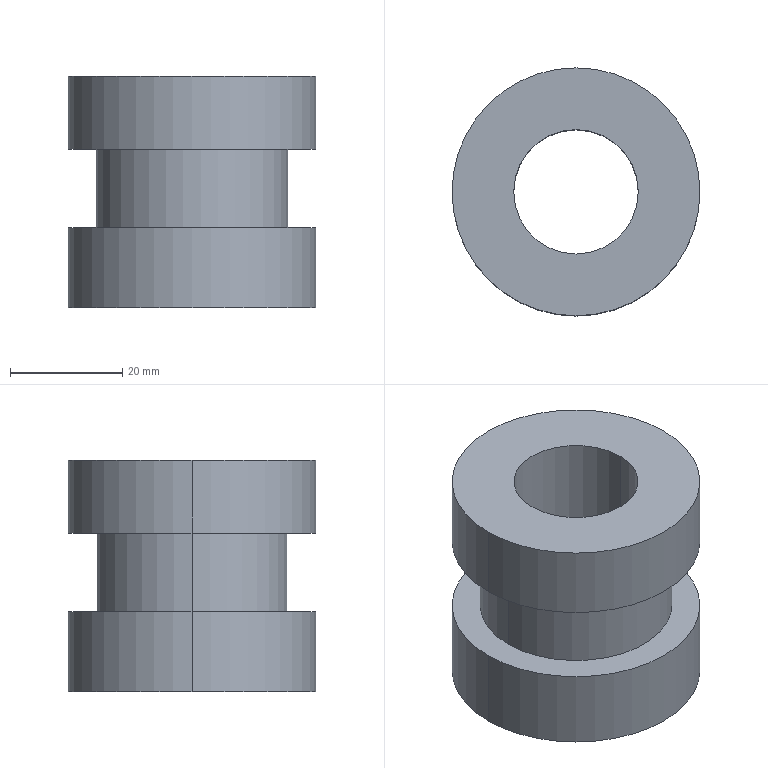Part | STEP file | 4-20.sldasm-Part-109 | 1 solid | 12 faces | box 44.22 x 44.22 x 41.275 mm | volume 38759 mm3 | cylinder 8 | plane 4 | commonest cylinder face diameters 44.22 x4 22.22 x2 34.22 x2
STEP:
#1=CARTESIAN_POINT('',(22.11,-584.45,-181.275));
#2=VERTEX_POINT('',#1);
#3=CARTESIAN_POINT('',(-22.11,-584.45,-181.275));
#4=VERTEX_POINT('',#3);
#5=CARTESIAN_POINT('',(0.,-584.45,-181.275));
#6=DIRECTION('',(0.,0.,1.));
#7=DIRECTION('',(1.,0.,0.));
#8=AXIS2_PLACEMENT_3D('',#5,#6,#7);
#9=CIRCLE('',#8,22.11);
#10=EDGE_CURVE('',#2,#4,#9,.T.);
#11=ORIENTED_EDGE('',*,*,#10,.T.);
#12=CARTESIAN_POINT('',(-22.11,-584.45,-167.));
#13=VERTEX_POINT('',#12);
#14=CARTESIAN_POINT('',(-22.11,-584.45,-179.));
#15=DIRECTION('',(0.,0.,1.));
#16=VECTOR('',#15,1000.);
#17=LINE('',#14,#16);
#18=EDGE_CURVE('',#4,#13,#17,.T.);
#19=ORIENTED_EDGE('',*,*,#18,.T.);
#20=CARTESIAN_POINT('',(22.11,-584.45,-167.));
#21=VERTEX_POINT('',#20);
#22=CARTESIAN_POINT('',(0.,-584.45,-167.));
#23=DIRECTION('',(0.,0.,1.));
#24=DIRECTION('',(-1.,0.,0.));
#25=AXIS2_PLACEMENT_3D('',#22,#23,#24);
#26=CIRCLE('',#25,22.11);
#27=EDGE_CURVE('',#21,#13,#26,.T.);
#28=ORIENTED_EDGE('',*,*,#27,.F.);
#29=CARTESIAN_POINT('',(22.11,-584.45,-179.));
#30=DIRECTION('',(0.,0.,1.));
#31=VECTOR('',#30,1000.);
#32=LINE('',#29,#31);
#33=EDGE_CURVE('',#2,#21,#32,.T.);
#34=ORIENTED_EDGE('',*,*,#33,.F.);
#35=EDGE_LOOP('',(#11,#19,#28,#34));
#36=FACE_OUTER_BOUND('',#35,.T.);
#37=CARTESIAN_POINT('',(0.,-584.45,-179.));
#38=DIRECTION('',(0.,0.,1.));
#39=DIRECTION('',(1.,0.,0.));
#40=AXIS2_PLACEMENT_3D('',#37,#38,#39);
#41=CYLINDRICAL_SURFACE('',#40,22.11);
#42=ADVANCED_FACE('',(#36),#41,.T.);
#43=CARTESIAN_POINT('',(-22.11,-584.45,-140.));
#44=VERTEX_POINT('',#43);
#45=CARTESIAN_POINT('',(22.11,-584.45,-140.));
#46=VERTEX_POINT('',#45);
#47=CARTESIAN_POINT('',(0.,-584.45,-140.));
#48=DIRECTION('',(0.,0.,-1.));
#49=DIRECTION('',(1.,0.,0.));
#50=AXIS2_PLACEMENT_3D('',#47,#48,#49);
#51=CIRCLE('',#50,22.11);
#52=EDGE_CURVE('',#44,#46,#51,.T.);
#53=ORIENTED_EDGE('',*,*,#52,.T.);
#54=CARTESIAN_POINT('',(22.11,-584.45,-153.));
#55=VERTEX_POINT('',#54);
#56=CARTESIAN_POINT('',(22.11,-584.45,-139.));
#57=DIRECTION('',(0.,0.,-1.));
#58=VECTOR('',#57,1000.);
#59=LINE('',#56,#58);
#60=EDGE_CURVE('',#46,#55,#59,.T.);
#61=ORIENTED_EDGE('',*,*,#60,.T.);
#62=CARTESIAN_POINT('',(-22.11,-584.45,-153.));
#63=VERTEX_POINT('',#62);
#64=CARTESIAN_POINT('',(0.,-584.45,-153.));
#65=DIRECTION('',(0.,0.,-1.));
#66=DIRECTION('',(1.,0.,0.));
#67=AXIS2_PLACEMENT_3D('',#64,#65,#66);
#68=CIRCLE('',#67,22.11);
#69=EDGE_CURVE('',#63,#55,#68,.T.);
#70=ORIENTED_EDGE('',*,*,#69,.F.);
#71=CARTESIAN_POINT('',(-22.11,-584.45,-139.));
#72=DIRECTION('',(0.,0.,-1.));
#73=VECTOR('',#72,1000.);
#74=LINE('',#71,#73);
#75=EDGE_CURVE('',#44,#63,#74,.T.);
#76=ORIENTED_EDGE('',*,*,#75,.F.);
#77=EDGE_LOOP('',(#53,#61,#70,#76));
#78=FACE_OUTER_BOUND('',#77,.T.);
#79=CARTESIAN_POINT('',(0.,-584.45,-139.));
#80=DIRECTION('',(0.,0.,-1.));
#81=DIRECTION('',(-1.,0.,0.));
#82=AXIS2_PLACEMENT_3D('',#79,#80,#81);
#83=CYLINDRICAL_SURFACE('',#82,22.11);
#84=ADVANCED_FACE('',(#78),#83,.T.);
#85=CARTESIAN_POINT('',(-11.11,-584.45,-181.275));
#86=VERTEX_POINT('',#85);
#87=CARTESIAN_POINT('',(11.11,-584.45,-181.275));
#88=VERTEX_POINT('',#87);
#89=CARTESIAN_POINT('',(0.,-584.45,-181.275));
#90=DIRECTION('',(0.,0.,1.));
#91=DIRECTION('',(1.,0.,0.));
#92=AXIS2_PLACEMENT_3D('',#89,#90,#91);
#93=CIRCLE('',#92,11.11);
#94=EDGE_CURVE('',#86,#88,#93,.T.);
#95=ORIENTED_EDGE('',*,*,#94,.F.);
#96=CARTESIAN_POINT('',(-11.11,-584.45,-140.));
#97=VERTEX_POINT('',#96);
#98=CARTESIAN_POINT('',(-11.11,-584.45,-168.9));
#99=DIRECTION('',(0.,0.,1.));
#100=VECTOR('',#99,1000.);
#101=LINE('',#98,#100);
#102=EDGE_CURVE('',#86,#97,#101,.T.);
#103=ORIENTED_EDGE('',*,*,#102,.T.);
#104=CARTESIAN_POINT('',(11.11,-584.45,-140.));
#105=VERTEX_POINT('',#104);
#106=CARTESIAN_POINT('',(0.,-584.45,-140.));
#107=DIRECTION('',(0.,0.,1.));
#108=DIRECTION('',(1.,0.,0.));
#109=AXIS2_PLACEMENT_3D('',#106,#107,#108);
#110=CIRCLE('',#109,11.11);
#111=EDGE_CURVE('',#97,#105,#110,.T.);
#112=ORIENTED_EDGE('',*,*,#111,.T.);
#113=CARTESIAN_POINT('',(11.11,-584.45,-168.9));
#114=DIRECTION('',(0.,0.,1.));
#115=VECTOR('',#114,1000.);
#116=LINE('',#113,#115);
#117=EDGE_CURVE('',#88,#105,#116,.T.);
#118=ORIENTED_EDGE('',*,*,#117,.F.);
#119=EDGE_LOOP('',(#95,#103,#112,#118));
#120=FACE_OUTER_BOUND('',#119,.T.);
#121=CARTESIAN_POINT('',(0.,-584.45,-168.9));
#122=DIRECTION('',(0.,0.,1.));
#123=DIRECTION('',(1.,0.,0.));
#124=AXIS2_PLACEMENT_3D('',#121,#122,#123);
#125=CYLINDRICAL_SURFACE('',#124,11.11);
#126=ADVANCED_FACE('',(#120),#125,.F.);
#127=CARTESIAN_POINT('',(-17.11,-584.45,-167.));
#128=VERTEX_POINT('',#127);
#129=CARTESIAN_POINT('',(17.11,-584.45,-167.));
#130=VERTEX_POINT('',#129);
#131=CARTESIAN_POINT('',(0.,-584.45,-167.));
#132=DIRECTION('',(0.,0.,-1.));
#133=DIRECTION('',(-1.,0.,0.));
#134=AXIS2_PLACEMENT_3D('',#131,#132,#133);
#135=CIRCLE('',#134,17.11);
#136=EDGE_CURVE('',#128,#130,#135,.T.);
#137=ORIENTED_EDGE('',*,*,#136,.F.);
#138=CARTESIAN_POINT('',(-17.11,-584.45,-153.));
#139=VERTEX_POINT('',#138);
#140=CARTESIAN_POINT('',(-17.11,-584.45,-168.9));
#141=DIRECTION('',(0.,0.,1.));
#142=VECTOR('',#141,1000.);
#143=LINE('',#140,#142);
#144=EDGE_CURVE('',#128,#139,#143,.T.);
#145=ORIENTED_EDGE('',*,*,#144,.T.);
#146=CARTESIAN_POINT('',(17.11,-584.45,-153.));
#147=VERTEX_POINT('',#146);
#148=CARTESIAN_POINT('',(0.,-584.45,-153.));
#149=DIRECTION('',(0.,0.,1.));
#150=DIRECTION('',(1.,0.,0.));
#151=AXIS2_PLACEMENT_3D('',#148,#149,#150);
#152=CIRCLE('',#151,17.11);
#153=EDGE_CURVE('',#147,#139,#152,.T.);
#154=ORIENTED_EDGE('',*,*,#153,.F.);
#155=CARTESIAN_POINT('',(17.11,-584.45,-168.9));
#156=DIRECTION('',(0.,0.,1.));
#157=VECTOR('',#156,1000.);
#158=LINE('',#155,#157);
#159=EDGE_CURVE('',#130,#147,#158,.T.);
#160=ORIENTED_EDGE('',*,*,#159,.F.);
#161=EDGE_LOOP('',(#137,#145,#154,#160));
#162=FACE_OUTER_BOUND('',#161,.T.);
#163=CARTESIAN_POINT('',(0.,-584.45,-168.9));
#164=DIRECTION('',(0.,0.,1.));
#165=DIRECTION('',(1.,0.,0.));
#166=AXIS2_PLACEMENT_3D('',#163,#164,#165);
#167=CYLINDRICAL_SURFACE('',#166,17.11);
#168=ADVANCED_FACE('',(#162),#167,.T.);
#169=ORIENTED_EDGE('',*,*,#144,.F.);
#170=CARTESIAN_POINT('',(0.,-584.45,-167.));
#171=DIRECTION('',(0.,0.,-1.));
#172=DIRECTION('',(-1.,0.,0.));
#173=AXIS2_PLACEMENT_3D('',#170,#171,#172);
#174=CIRCLE('',#173,17.11);
#175=EDGE_CURVE('',#130,#128,#174,.T.);
#176=ORIENTED_EDGE('',*,*,#175,.F.);
#177=ORIENTED_EDGE('',*,*,#159,.T.);
#178=CARTESIAN_POINT('',(0.,-584.45,-153.));
#179=DIRECTION('',(0.,0.,1.));
#180=DIRECTION('',(1.,0.,0.));
#181=AXIS2_PLACEMENT_3D('',#178,#179,#180);
#182=CIRCLE('',#181,17.11);
#183=EDGE_CURVE('',#139,#147,#182,.T.);
#184=ORIENTED_EDGE('',*,*,#183,.F.);
#185=EDGE_LOOP('',(#169,#176,#177,#184));
#186=FACE_OUTER_BOUND('',#185,.T.);
#187=CARTESIAN_POINT('',(0.,-584.45,-168.9));
#188=DIRECTION('',(0.,0.,1.));
#189=DIRECTION('',(1.,0.,0.));
#190=AXIS2_PLACEMENT_3D('',#187,#188,#189);
#191=CYLINDRICAL_SURFACE('',#190,17.11);
#192=ADVANCED_FACE('',(#186),#191,.T.);
#193=ORIENTED_EDGE('',*,*,#52,.F.);
#194=CARTESIAN_POINT('',(0.,-584.45,-140.));
#195=DIRECTION('',(0.,0.,-1.));
#196=DIRECTION('',(1.,0.,0.));
#197=AXIS2_PLACEMENT_3D('',#194,#195,#196);
#198=CIRCLE('',#197,22.11);
#199=EDGE_CURVE('',#46,#44,#198,.T.);
#200=ORIENTED_EDGE('',*,*,#199,.F.);
#201=EDGE_LOOP('',(#193,#200));
#202=FACE_OUTER_BOUND('',#201,.T.);
#203=CARTESIAN_POINT('',(0.,-584.45,-140.));
#204=DIRECTION('',(0.,0.,1.));
#205=DIRECTION('',(1.,0.,0.));
#206=AXIS2_PLACEMENT_3D('',#203,#204,#205);
#207=CIRCLE('',#206,11.11);
#208=EDGE_CURVE('',#105,#97,#207,.T.);
#209=ORIENTED_EDGE('',*,*,#208,.F.);
#210=ORIENTED_EDGE('',*,*,#111,.F.);
#211=EDGE_LOOP('',(#209,#210));
#212=FACE_BOUND('',#211,.T.);
#213=CARTESIAN_POINT('',(285.75,-707.7,-140.));
#214=DIRECTION('',(0.,0.,1.));
#215=DIRECTION('',(1.,0.,0.));
#216=AXIS2_PLACEMENT_3D('',#213,#214,#215);
#217=PLANE('',#216);
#218=ADVANCED_FACE('',(#202,#212),#217,.T.);
#219=ORIENTED_EDGE('',*,*,#10,.F.);
#220=CARTESIAN_POINT('',(0.,-584.45,-181.275));
#221=DIRECTION('',(0.,0.,1.));
#222=DIRECTION('',(1.,0.,0.));
#223=AXIS2_PLACEMENT_3D('',#220,#221,#222);
#224=CIRCLE('',#223,22.11);
#225=EDGE_CURVE('',#4,#2,#224,.T.);
#226=ORIENTED_EDGE('',*,*,#225,.F.);
#227=EDGE_LOOP('',(#219,#226));
#228=FACE_OUTER_BOUND('',#227,.T.);
#229=CARTESIAN_POINT('',(0.,-584.45,-181.275));
#230=DIRECTION('',(0.,0.,1.));
#231=DIRECTION('',(1.,0.,0.));
#232=AXIS2_PLACEMENT_3D('',#229,#230,#231);
#233=CIRCLE('',#232,11.11);
#234=EDGE_CURVE('',#88,#86,#233,.T.);
#235=ORIENTED_EDGE('',*,*,#234,.T.);
#236=ORIENTED_EDGE('',*,*,#94,.T.);
#237=EDGE_LOOP('',(#235,#236));
#238=FACE_BOUND('',#237,.T.);
#239=CARTESIAN_POINT('',(-346.067,-548.4,-181.275));
#240=DIRECTION('',(0.,0.,1.));
#241=DIRECTION('',(0.,-1.,0.));
#242=AXIS2_PLACEMENT_3D('',#239,#240,#241);
#243=PLANE('',#242);
#244=ADVANCED_FACE('',(#228,#238),#243,.F.);
#245=ORIENTED_EDGE('',*,*,#102,.F.);
#246=ORIENTED_EDGE('',*,*,#234,.F.);
#247=ORIENTED_EDGE('',*,*,#117,.T.);
#248=ORIENTED_EDGE('',*,*,#208,.T.);
#249=EDGE_LOOP('',(#245,#246,#247,#248));
#250=FACE_OUTER_BOUND('',#249,.T.);
#251=CARTESIAN_POINT('',(0.,-584.45,-168.9));
#252=DIRECTION('',(0.,0.,1.));
#253=DIRECTION('',(1.,0.,0.));
#254=AXIS2_PLACEMENT_3D('',#251,#252,#253);
#255=CYLINDRICAL_SURFACE('',#254,11.11);
#256=ADVANCED_FACE('',(#250),#255,.F.);
#257=ORIENTED_EDGE('',*,*,#60,.F.);
#258=ORIENTED_EDGE('',*,*,#199,.T.);
#259=ORIENTED_EDGE('',*,*,#75,.T.);
#260=CARTESIAN_POINT('',(0.,-584.45,-153.));
#261=DIRECTION('',(0.,0.,-1.));
#262=DIRECTION('',(1.,0.,0.));
#263=AXIS2_PLACEMENT_3D('',#260,#261,#262);
#264=CIRCLE('',#263,22.11);
#265=EDGE_CURVE('',#55,#63,#264,.T.);
#266=ORIENTED_EDGE('',*,*,#265,.F.);
#267=EDGE_LOOP('',(#257,#258,#259,#266));
#268=FACE_OUTER_BOUND('',#267,.T.);
#269=CARTESIAN_POINT('',(0.,-584.45,-139.));
#270=DIRECTION('',(0.,0.,-1.));
#271=DIRECTION('',(-1.,0.,0.));
#272=AXIS2_PLACEMENT_3D('',#269,#270,#271);
#273=CYLINDRICAL_SURFACE('',#272,22.11);
#274=ADVANCED_FACE('',(#268),#273,.T.);
#275=ORIENTED_EDGE('',*,*,#153,.T.);
#276=ORIENTED_EDGE('',*,*,#183,.T.);
#277=EDGE_LOOP('',(#275,#276));
#278=FACE_BOUND('',#277,.T.);
#279=ORIENTED_EDGE('',*,*,#69,.T.);
#280=ORIENTED_EDGE('',*,*,#265,.T.);
#281=EDGE_LOOP('',(#279,#280));
#282=FACE_OUTER_BOUND('',#281,.T.);
#283=CARTESIAN_POINT('',(0.,-584.45,-153.));
#284=DIRECTION('',(0.,0.,1.));
#285=DIRECTION('',(1.,0.,0.));
#286=AXIS2_PLACEMENT_3D('',#283,#284,#285);
#287=PLANE('',#286);
#288=ADVANCED_FACE('',(#278,#282),#287,.F.);
#289=ORIENTED_EDGE('',*,*,#18,.F.);
#290=ORIENTED_EDGE('',*,*,#225,.T.);
#291=ORIENTED_EDGE('',*,*,#33,.T.);
#292=CARTESIAN_POINT('',(0.,-584.45,-167.));
#293=DIRECTION('',(0.,0.,1.));
#294=DIRECTION('',(-1.,0.,0.));
#295=AXIS2_PLACEMENT_3D('',#292,#293,#294);
#296=CIRCLE('',#295,22.11);
#297=EDGE_CURVE('',#13,#21,#296,.T.);
#298=ORIENTED_EDGE('',*,*,#297,.F.);
#299=EDGE_LOOP('',(#289,#290,#291,#298));
#300=FACE_OUTER_BOUND('',#299,.T.);
#301=CARTESIAN_POINT('',(0.,-584.45,-179.));
#302=DIRECTION('',(0.,0.,1.));
#303=DIRECTION('',(1.,0.,0.));
#304=AXIS2_PLACEMENT_3D('',#301,#302,#303);
#305=CYLINDRICAL_SURFACE('',#304,22.11);
#306=ADVANCED_FACE('',(#300),#305,.T.);
#307=ORIENTED_EDGE('',*,*,#175,.T.);
#308=ORIENTED_EDGE('',*,*,#136,.T.);
#309=EDGE_LOOP('',(#307,#308));
#310=FACE_BOUND('',#309,.T.);
#311=ORIENTED_EDGE('',*,*,#27,.T.);
#312=ORIENTED_EDGE('',*,*,#297,.T.);
#313=EDGE_LOOP('',(#311,#312));
#314=FACE_OUTER_BOUND('',#313,.T.);
#315=CARTESIAN_POINT('',(0.,-584.45,-167.));
#316=DIRECTION('',(0.,0.,-1.));
#317=DIRECTION('',(-1.,0.,0.));
#318=AXIS2_PLACEMENT_3D('',#315,#316,#317);
#319=PLANE('',#318);
#320=ADVANCED_FACE('',(#310,#314),#319,.F.);
#321=CLOSED_SHELL('',(#42,#84,#126,#168,#192,#218,#244,#256,#274,#288,#306,#320));
#322=MANIFOLD_SOLID_BREP('',#321);
#323=CARTESIAN_POINT('',(0.,0.,0.));
#324=DIRECTION('',(0.,0.,1.));
#325=DIRECTION('',(1.,0.,0.));
#326=AXIS2_PLACEMENT_3D('',#323,#324,#325);
#327=(LENGTH_UNIT()NAMED_UNIT(*)SI_UNIT(.MILLI.,.METRE.));
#328=UNCERTAINTY_MEASURE_WITH_UNIT(LENGTH_MEASURE(0.00001),#327,'','');
#329=(NAMED_UNIT(*)PLANE_ANGLE_UNIT()SI_UNIT($,.RADIAN.));
#330=(NAMED_UNIT(*)SI_UNIT($,.STERADIAN.)SOLID_ANGLE_UNIT());
#331=(GEOMETRIC_REPRESENTATION_CONTEXT(3)GLOBAL_UNCERTAINTY_ASSIGNED_CONTEXT((#328))GLOBAL_UNIT_ASSIGNED_CONTEXT((#327,#329,#330))REPRESENTATION_CONTEXT('',''));
#332=ADVANCED_BREP_SHAPE_REPRESENTATION('',(#322,#326),#331);